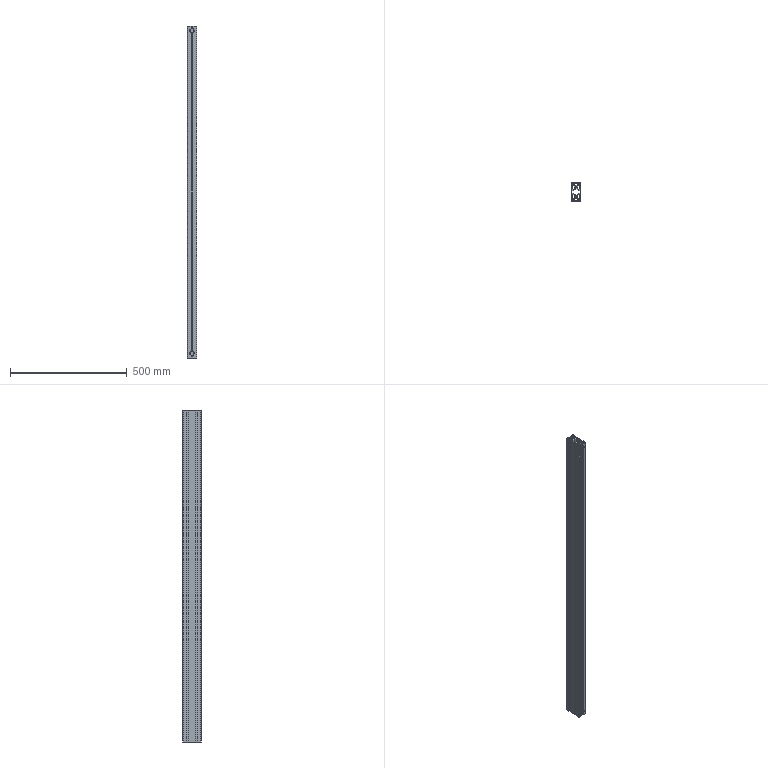Part | STEP file | 09-09 aluminium profile 4080-1420 | 1 solid | 170 faces | box 40 x 80 x 1420 mm | volume 1707613 mm3 | plane 134 | cylinder 36 | commonest cylinder face diameters 18.5 x20 5 x8 4 x4 6.7 x4